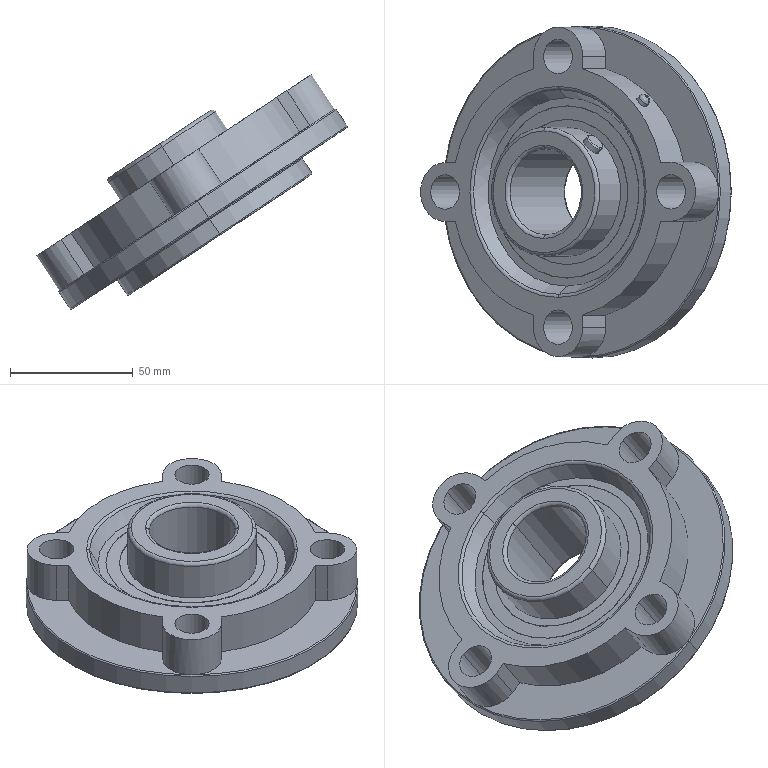Part | STEP file | HL4GZ-1.862.293 (pillow block bearing) | 1 solid | 90 faces | box 126.394 x 135 x 95.577 mm | volume 264041 mm3 | cylinder 37 | torus 24 | plane 23 | cone 4 | spline 2 | commonest cylinder face diameters 14.026 x8 23.974 x5 52.5 x4 103.013 x4 5 x2 8 x2